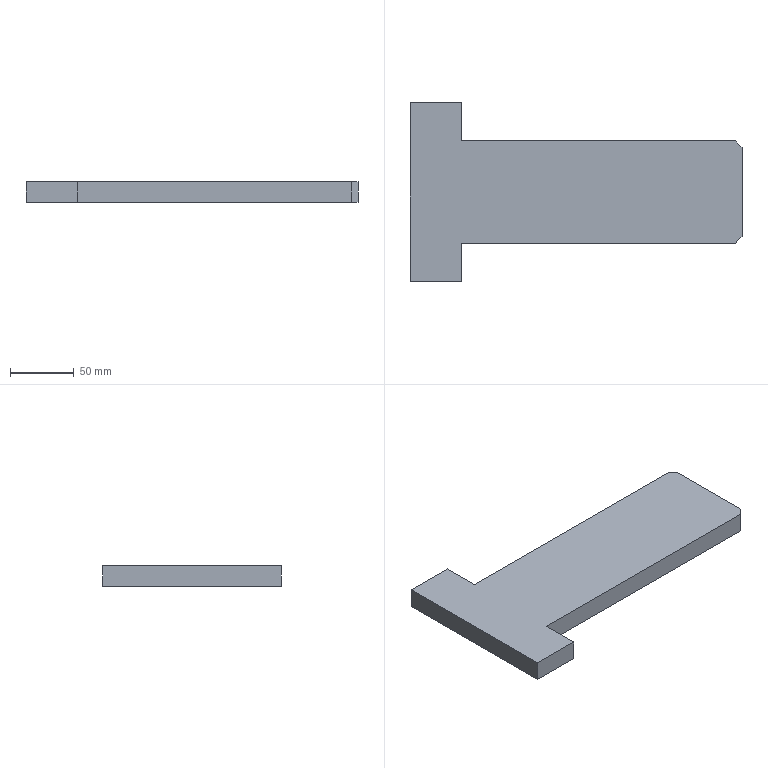Part | NX | features 梁销挡板 2 | 1 solid | 12 faces | box 260 x 140 x 16 mm | volume 370800 mm3 | plane 12
STEP:
#1=CARTESIAN_POINT('',(-54.422,70.,0.));
#2=VERTEX_POINT('',#1);
#3=CARTESIAN_POINT('',(-94.422,70.,0.));
#4=VERTEX_POINT('',#3);
#5=CARTESIAN_POINT('',(-94.422,70.,0.));
#6=DIRECTION('',(-1.,0.,0.));
#7=VECTOR('',#6,1000.);
#8=LINE('',#5,#7);
#9=EDGE_CURVE('',#2,#4,#8,.T.);
#10=ORIENTED_EDGE('',*,*,#9,.T.);
#11=CARTESIAN_POINT('',(-94.422,70.,16.));
#12=VERTEX_POINT('',#11);
#13=CARTESIAN_POINT('',(-94.422,70.,16.));
#14=DIRECTION('',(0.,0.,-1.));
#15=VECTOR('',#14,1000.);
#16=LINE('',#13,#15);
#17=EDGE_CURVE('',#12,#4,#16,.T.);
#18=ORIENTED_EDGE('',*,*,#17,.F.);
#19=CARTESIAN_POINT('',(-54.422,70.,16.));
#20=VERTEX_POINT('',#19);
#21=CARTESIAN_POINT('',(-94.422,70.,16.));
#22=DIRECTION('',(-1.,0.,0.));
#23=VECTOR('',#22,1000.);
#24=LINE('',#21,#23);
#25=EDGE_CURVE('',#20,#12,#24,.T.);
#26=ORIENTED_EDGE('',*,*,#25,.F.);
#27=CARTESIAN_POINT('',(-54.422,70.,16.));
#28=DIRECTION('',(0.,0.,-1.));
#29=VECTOR('',#28,1000.);
#30=LINE('',#27,#29);
#31=EDGE_CURVE('',#20,#2,#30,.T.);
#32=ORIENTED_EDGE('',*,*,#31,.T.);
#33=EDGE_LOOP('',(#10,#18,#26,#32));
#34=FACE_BOUND('',#33,.T.);
#35=CARTESIAN_POINT('',(-94.422,70.,16.));
#36=DIRECTION('',(0.,-1.,0.));
#37=DIRECTION('',(0.,0.,-1.));
#38=AXIS2_PLACEMENT_3D('',#35,#36,#37);
#39=PLANE('',#38);
#40=ADVANCED_FACE('',(#34),#39,.F.);
#41=CARTESIAN_POINT('',(-94.422,-70.,0.));
#42=VERTEX_POINT('',#41);
#43=CARTESIAN_POINT('',(-94.422,-70.,0.));
#44=DIRECTION('',(0.,-1.,0.));
#45=VECTOR('',#44,1000.);
#46=LINE('',#43,#45);
#47=EDGE_CURVE('',#4,#42,#46,.T.);
#48=ORIENTED_EDGE('',*,*,#47,.T.);
#49=CARTESIAN_POINT('',(-94.422,-70.,16.));
#50=VERTEX_POINT('',#49);
#51=CARTESIAN_POINT('',(-94.422,-70.,16.));
#52=DIRECTION('',(0.,0.,-1.));
#53=VECTOR('',#52,1000.);
#54=LINE('',#51,#53);
#55=EDGE_CURVE('',#50,#42,#54,.T.);
#56=ORIENTED_EDGE('',*,*,#55,.F.);
#57=CARTESIAN_POINT('',(-94.422,-70.,16.));
#58=DIRECTION('',(0.,-1.,0.));
#59=VECTOR('',#58,1000.);
#60=LINE('',#57,#59);
#61=EDGE_CURVE('',#12,#50,#60,.T.);
#62=ORIENTED_EDGE('',*,*,#61,.F.);
#63=ORIENTED_EDGE('',*,*,#17,.T.);
#64=EDGE_LOOP('',(#48,#56,#62,#63));
#65=FACE_BOUND('',#64,.T.);
#66=CARTESIAN_POINT('',(-94.422,-70.,16.));
#67=DIRECTION('',(1.,0.,0.));
#68=DIRECTION('',(0.,0.,-1.));
#69=AXIS2_PLACEMENT_3D('',#66,#67,#68);
#70=PLANE('',#69);
#71=ADVANCED_FACE('',(#65),#70,.F.);
#72=CARTESIAN_POINT('',(-54.422,-70.,0.));
#73=VERTEX_POINT('',#72);
#74=CARTESIAN_POINT('',(-94.422,-70.,0.));
#75=DIRECTION('',(1.,0.,0.));
#76=VECTOR('',#75,1000.);
#77=LINE('',#74,#76);
#78=EDGE_CURVE('',#42,#73,#77,.T.);
#79=ORIENTED_EDGE('',*,*,#78,.T.);
#80=CARTESIAN_POINT('',(-54.422,-70.,16.));
#81=VERTEX_POINT('',#80);
#82=CARTESIAN_POINT('',(-54.422,-70.,16.));
#83=DIRECTION('',(0.,0.,-1.));
#84=VECTOR('',#83,1000.);
#85=LINE('',#82,#84);
#86=EDGE_CURVE('',#81,#73,#85,.T.);
#87=ORIENTED_EDGE('',*,*,#86,.F.);
#88=CARTESIAN_POINT('',(-94.422,-70.,16.));
#89=DIRECTION('',(1.,0.,0.));
#90=VECTOR('',#89,1000.);
#91=LINE('',#88,#90);
#92=EDGE_CURVE('',#50,#81,#91,.T.);
#93=ORIENTED_EDGE('',*,*,#92,.F.);
#94=ORIENTED_EDGE('',*,*,#55,.T.);
#95=EDGE_LOOP('',(#79,#87,#93,#94));
#96=FACE_BOUND('',#95,.T.);
#97=CARTESIAN_POINT('',(-94.422,-70.,16.));
#98=DIRECTION('',(0.,1.,0.));
#99=DIRECTION('',(0.,0.,1.));
#100=AXIS2_PLACEMENT_3D('',#97,#98,#99);
#101=PLANE('',#100);
#102=ADVANCED_FACE('',(#96),#101,.F.);
#103=CARTESIAN_POINT('',(-54.422,-40.,0.));
#104=VERTEX_POINT('',#103);
#105=CARTESIAN_POINT('',(-54.422,-70.,0.));
#106=DIRECTION('',(0.,1.,0.));
#107=VECTOR('',#106,1000.);
#108=LINE('',#105,#107);
#109=EDGE_CURVE('',#73,#104,#108,.T.);
#110=ORIENTED_EDGE('',*,*,#109,.T.);
#111=CARTESIAN_POINT('',(-54.422,-40.,16.));
#112=VERTEX_POINT('',#111);
#113=CARTESIAN_POINT('',(-54.422,-40.,16.));
#114=DIRECTION('',(0.,0.,-1.));
#115=VECTOR('',#114,1000.);
#116=LINE('',#113,#115);
#117=EDGE_CURVE('',#112,#104,#116,.T.);
#118=ORIENTED_EDGE('',*,*,#117,.F.);
#119=CARTESIAN_POINT('',(-54.422,-70.,16.));
#120=DIRECTION('',(0.,1.,0.));
#121=VECTOR('',#120,1000.);
#122=LINE('',#119,#121);
#123=EDGE_CURVE('',#81,#112,#122,.T.);
#124=ORIENTED_EDGE('',*,*,#123,.F.);
#125=ORIENTED_EDGE('',*,*,#86,.T.);
#126=EDGE_LOOP('',(#110,#118,#124,#125));
#127=FACE_BOUND('',#126,.T.);
#128=CARTESIAN_POINT('',(-54.422,-70.,16.));
#129=DIRECTION('',(-1.,0.,0.));
#130=DIRECTION('',(0.,0.,1.));
#131=AXIS2_PLACEMENT_3D('',#128,#129,#130);
#132=PLANE('',#131);
#133=ADVANCED_FACE('',(#127),#132,.F.);
#134=CARTESIAN_POINT('',(160.578,-40.,0.));
#135=VERTEX_POINT('',#134);
#136=CARTESIAN_POINT('',(-54.422,-40.,0.));
#137=DIRECTION('',(1.,0.,0.));
#138=VECTOR('',#137,1000.);
#139=LINE('',#136,#138);
#140=EDGE_CURVE('',#104,#135,#139,.T.);
#141=ORIENTED_EDGE('',*,*,#140,.T.);
#142=CARTESIAN_POINT('',(160.578,-40.,16.));
#143=VERTEX_POINT('',#142);
#144=CARTESIAN_POINT('',(160.578,-40.,16.));
#145=DIRECTION('',(0.,0.,-1.));
#146=VECTOR('',#145,1000.);
#147=LINE('',#144,#146);
#148=EDGE_CURVE('',#143,#135,#147,.T.);
#149=ORIENTED_EDGE('',*,*,#148,.F.);
#150=CARTESIAN_POINT('',(-54.422,-40.,16.));
#151=DIRECTION('',(1.,0.,0.));
#152=VECTOR('',#151,1000.);
#153=LINE('',#150,#152);
#154=EDGE_CURVE('',#112,#143,#153,.T.);
#155=ORIENTED_EDGE('',*,*,#154,.F.);
#156=ORIENTED_EDGE('',*,*,#117,.T.);
#157=EDGE_LOOP('',(#141,#149,#155,#156));
#158=FACE_BOUND('',#157,.T.);
#159=CARTESIAN_POINT('',(-54.422,-40.,16.));
#160=DIRECTION('',(0.,1.,0.));
#161=DIRECTION('',(0.,0.,1.));
#162=AXIS2_PLACEMENT_3D('',#159,#160,#161);
#163=PLANE('',#162);
#164=ADVANCED_FACE('',(#158),#163,.F.);
#165=CARTESIAN_POINT('',(165.578,-35.,0.));
#166=VERTEX_POINT('',#165);
#167=CARTESIAN_POINT('',(160.578,-40.,0.));
#168=DIRECTION('',(0.7071,0.7071,0.));
#169=VECTOR('',#168,1000.);
#170=LINE('',#167,#169);
#171=EDGE_CURVE('',#135,#166,#170,.T.);
#172=ORIENTED_EDGE('',*,*,#171,.T.);
#173=CARTESIAN_POINT('',(165.578,-35.,16.));
#174=VERTEX_POINT('',#173);
#175=CARTESIAN_POINT('',(165.578,-35.,16.));
#176=DIRECTION('',(0.,0.,-1.));
#177=VECTOR('',#176,1000.);
#178=LINE('',#175,#177);
#179=EDGE_CURVE('',#174,#166,#178,.T.);
#180=ORIENTED_EDGE('',*,*,#179,.F.);
#181=CARTESIAN_POINT('',(160.578,-40.,16.));
#182=DIRECTION('',(0.7071,0.7071,0.));
#183=VECTOR('',#182,1000.);
#184=LINE('',#181,#183);
#185=EDGE_CURVE('',#143,#174,#184,.T.);
#186=ORIENTED_EDGE('',*,*,#185,.F.);
#187=ORIENTED_EDGE('',*,*,#148,.T.);
#188=EDGE_LOOP('',(#172,#180,#186,#187));
#189=FACE_BOUND('',#188,.T.);
#190=CARTESIAN_POINT('',(160.578,-40.,16.));
#191=DIRECTION('',(-0.7071,0.7071,0.));
#192=DIRECTION('',(-0.7071,-0.7071,0.));
#193=AXIS2_PLACEMENT_3D('',#190,#191,#192);
#194=PLANE('',#193);
#195=ADVANCED_FACE('',(#189),#194,.F.);
#196=CARTESIAN_POINT('',(165.578,35.,0.));
#197=VERTEX_POINT('',#196);
#198=CARTESIAN_POINT('',(165.578,35.,0.));
#199=DIRECTION('',(0.,1.,0.));
#200=VECTOR('',#199,1000.);
#201=LINE('',#198,#200);
#202=EDGE_CURVE('',#166,#197,#201,.T.);
#203=ORIENTED_EDGE('',*,*,#202,.T.);
#204=CARTESIAN_POINT('',(165.578,35.,16.));
#205=VERTEX_POINT('',#204);
#206=CARTESIAN_POINT('',(165.578,35.,16.));
#207=DIRECTION('',(0.,0.,-1.));
#208=VECTOR('',#207,1000.);
#209=LINE('',#206,#208);
#210=EDGE_CURVE('',#205,#197,#209,.T.);
#211=ORIENTED_EDGE('',*,*,#210,.F.);
#212=CARTESIAN_POINT('',(165.578,35.,16.));
#213=DIRECTION('',(0.,1.,0.));
#214=VECTOR('',#213,1000.);
#215=LINE('',#212,#214);
#216=EDGE_CURVE('',#174,#205,#215,.T.);
#217=ORIENTED_EDGE('',*,*,#216,.F.);
#218=ORIENTED_EDGE('',*,*,#179,.T.);
#219=EDGE_LOOP('',(#203,#211,#217,#218));
#220=FACE_BOUND('',#219,.T.);
#221=CARTESIAN_POINT('',(165.578,35.,16.));
#222=DIRECTION('',(-1.,0.,0.));
#223=DIRECTION('',(0.,0.,1.));
#224=AXIS2_PLACEMENT_3D('',#221,#222,#223);
#225=PLANE('',#224);
#226=ADVANCED_FACE('',(#220),#225,.F.);
#227=CARTESIAN_POINT('',(160.578,40.,0.));
#228=VERTEX_POINT('',#227);
#229=CARTESIAN_POINT('',(160.578,40.,0.));
#230=DIRECTION('',(-0.7071,0.7071,0.));
#231=VECTOR('',#230,1000.);
#232=LINE('',#229,#231);
#233=EDGE_CURVE('',#197,#228,#232,.T.);
#234=ORIENTED_EDGE('',*,*,#233,.T.);
#235=CARTESIAN_POINT('',(160.578,40.,16.));
#236=VERTEX_POINT('',#235);
#237=CARTESIAN_POINT('',(160.578,40.,16.));
#238=DIRECTION('',(0.,0.,-1.));
#239=VECTOR('',#238,1000.);
#240=LINE('',#237,#239);
#241=EDGE_CURVE('',#236,#228,#240,.T.);
#242=ORIENTED_EDGE('',*,*,#241,.F.);
#243=CARTESIAN_POINT('',(160.578,40.,16.));
#244=DIRECTION('',(-0.7071,0.7071,0.));
#245=VECTOR('',#244,1000.);
#246=LINE('',#243,#245);
#247=EDGE_CURVE('',#205,#236,#246,.T.);
#248=ORIENTED_EDGE('',*,*,#247,.F.);
#249=ORIENTED_EDGE('',*,*,#210,.T.);
#250=EDGE_LOOP('',(#234,#242,#248,#249));
#251=FACE_BOUND('',#250,.T.);
#252=CARTESIAN_POINT('',(160.578,40.,16.));
#253=DIRECTION('',(-0.7071,-0.7071,0.));
#254=DIRECTION('',(0.7071,-0.7071,0.));
#255=AXIS2_PLACEMENT_3D('',#252,#253,#254);
#256=PLANE('',#255);
#257=ADVANCED_FACE('',(#251),#256,.F.);
#258=CARTESIAN_POINT('',(-54.422,40.,0.));
#259=VERTEX_POINT('',#258);
#260=CARTESIAN_POINT('',(-54.422,40.,0.));
#261=DIRECTION('',(-1.,0.,0.));
#262=VECTOR('',#261,1000.);
#263=LINE('',#260,#262);
#264=EDGE_CURVE('',#228,#259,#263,.T.);
#265=ORIENTED_EDGE('',*,*,#264,.T.);
#266=CARTESIAN_POINT('',(-54.422,40.,16.));
#267=VERTEX_POINT('',#266);
#268=CARTESIAN_POINT('',(-54.422,40.,16.));
#269=DIRECTION('',(0.,0.,-1.));
#270=VECTOR('',#269,1000.);
#271=LINE('',#268,#270);
#272=EDGE_CURVE('',#267,#259,#271,.T.);
#273=ORIENTED_EDGE('',*,*,#272,.F.);
#274=CARTESIAN_POINT('',(-54.422,40.,16.));
#275=DIRECTION('',(-1.,0.,0.));
#276=VECTOR('',#275,1000.);
#277=LINE('',#274,#276);
#278=EDGE_CURVE('',#236,#267,#277,.T.);
#279=ORIENTED_EDGE('',*,*,#278,.F.);
#280=ORIENTED_EDGE('',*,*,#241,.T.);
#281=EDGE_LOOP('',(#265,#273,#279,#280));
#282=FACE_BOUND('',#281,.T.);
#283=CARTESIAN_POINT('',(-54.422,40.,16.));
#284=DIRECTION('',(0.,-1.,0.));
#285=DIRECTION('',(0.,0.,-1.));
#286=AXIS2_PLACEMENT_3D('',#283,#284,#285);
#287=PLANE('',#286);
#288=ADVANCED_FACE('',(#282),#287,.F.);
#289=CARTESIAN_POINT('',(-54.422,70.,0.));
#290=DIRECTION('',(0.,1.,0.));
#291=VECTOR('',#290,1000.);
#292=LINE('',#289,#291);
#293=EDGE_CURVE('',#259,#2,#292,.T.);
#294=ORIENTED_EDGE('',*,*,#293,.T.);
#295=ORIENTED_EDGE('',*,*,#31,.F.);
#296=CARTESIAN_POINT('',(-54.422,70.,16.));
#297=DIRECTION('',(0.,1.,0.));
#298=VECTOR('',#297,1000.);
#299=LINE('',#296,#298);
#300=EDGE_CURVE('',#267,#20,#299,.T.);
#301=ORIENTED_EDGE('',*,*,#300,.F.);
#302=ORIENTED_EDGE('',*,*,#272,.T.);
#303=EDGE_LOOP('',(#294,#295,#301,#302));
#304=FACE_BOUND('',#303,.T.);
#305=CARTESIAN_POINT('',(-54.422,70.,16.));
#306=DIRECTION('',(-1.,0.,0.));
#307=DIRECTION('',(0.,0.,1.));
#308=AXIS2_PLACEMENT_3D('',#305,#306,#307);
#309=PLANE('',#308);
#310=ADVANCED_FACE('',(#304),#309,.F.);
#311=ORIENTED_EDGE('',*,*,#25,.T.);
#312=ORIENTED_EDGE('',*,*,#61,.T.);
#313=ORIENTED_EDGE('',*,*,#92,.T.);
#314=ORIENTED_EDGE('',*,*,#123,.T.);
#315=ORIENTED_EDGE('',*,*,#154,.T.);
#316=ORIENTED_EDGE('',*,*,#185,.T.);
#317=ORIENTED_EDGE('',*,*,#216,.T.);
#318=ORIENTED_EDGE('',*,*,#247,.T.);
#319=ORIENTED_EDGE('',*,*,#278,.T.);
#320=ORIENTED_EDGE('',*,*,#300,.T.);
#321=EDGE_LOOP('',(#311,#312,#313,#314,#315,#316,#317,#318,#319,#320));
#322=FACE_BOUND('',#321,.T.);
#323=CARTESIAN_POINT('',(-54.422,70.,16.));
#324=DIRECTION('',(0.,0.,-1.));
#325=DIRECTION('',(-1.,0.,0.));
#326=AXIS2_PLACEMENT_3D('',#323,#324,#325);
#327=PLANE('',#326);
#328=ADVANCED_FACE('',(#322),#327,.F.);
#329=ORIENTED_EDGE('',*,*,#9,.F.);
#330=ORIENTED_EDGE('',*,*,#293,.F.);
#331=ORIENTED_EDGE('',*,*,#264,.F.);
#332=ORIENTED_EDGE('',*,*,#233,.F.);
#333=ORIENTED_EDGE('',*,*,#202,.F.);
#334=ORIENTED_EDGE('',*,*,#171,.F.);
#335=ORIENTED_EDGE('',*,*,#140,.F.);
#336=ORIENTED_EDGE('',*,*,#109,.F.);
#337=ORIENTED_EDGE('',*,*,#78,.F.);
#338=ORIENTED_EDGE('',*,*,#47,.F.);
#339=EDGE_LOOP('',(#329,#330,#331,#332,#333,#334,#335,#336,#337,#338));
#340=FACE_BOUND('',#339,.T.);
#341=CARTESIAN_POINT('',(-54.422,70.,0.));
#342=DIRECTION('',(0.,0.,-1.));
#343=DIRECTION('',(-1.,0.,0.));
#344=AXIS2_PLACEMENT_3D('',#341,#342,#343);
#345=PLANE('',#344);
#346=ADVANCED_FACE('',(#340),#345,.T.);
#347=CLOSED_SHELL('',(#40,#71,#102,#133,#164,#195,#226,#257,#288,#310,#328,#346));
#348=MANIFOLD_SOLID_BREP('',#347);
#349=(LENGTH_UNIT()NAMED_UNIT(*)SI_UNIT(.MILLI.,.METRE.));
#350=UNCERTAINTY_MEASURE_WITH_UNIT(LENGTH_MEASURE(0.00001),#349,'','');
#351=(NAMED_UNIT(*)PLANE_ANGLE_UNIT()SI_UNIT($,.RADIAN.));
#352=(NAMED_UNIT(*)SI_UNIT($,.STERADIAN.)SOLID_ANGLE_UNIT());
#353=(GEOMETRIC_REPRESENTATION_CONTEXT(3)GLOBAL_UNCERTAINTY_ASSIGNED_CONTEXT((#350))GLOBAL_UNIT_ASSIGNED_CONTEXT((#349,#351,#352))REPRESENTATION_CONTEXT('',''));
#354=ADVANCED_BREP_SHAPE_REPRESENTATION('',(#348),#353);